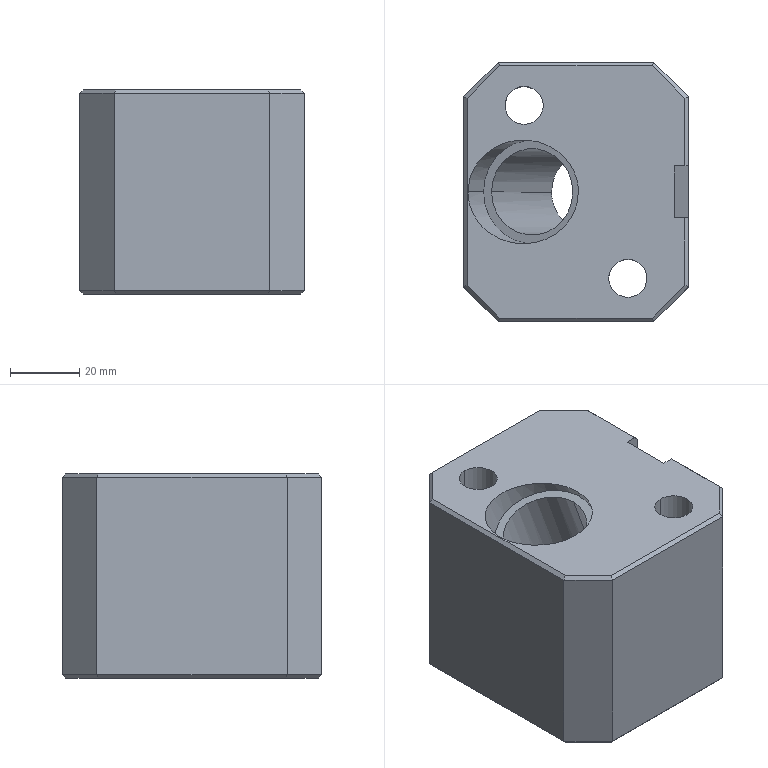Part | Creo | 3 solids | 49 faces | box 65 x 75 x 59 mm | volume 228073 mm3 | plane 33 | cylinder 16 | commonest cylinder face diameters 11 x4 18 x4 11.98 x2 12 x2 25 x2 30 x2
STEP:
#1=CARTESIAN_POINT('',(284.936,-85.497,48.));
#2=VERTEX_POINT('',#1);
#3=CARTESIAN_POINT('',(274.936,-75.497,48.));
#4=VERTEX_POINT('',#3);
#5=CARTESIAN_POINT('',(284.936,-85.497,48.));
#6=DIRECTION('',(-0.7071,0.7071,0.));
#7=VECTOR('',#6,14.142);
#8=LINE('',#5,#7);
#9=EDGE_CURVE('',#2,#4,#8,.T.);
#10=ORIENTED_EDGE('',*,*,#9,.T.);
#11=CARTESIAN_POINT('',(274.936,-75.497,-9.));
#12=VERTEX_POINT('',#11);
#13=CARTESIAN_POINT('',(274.936,-75.497,-9.));
#14=DIRECTION('',(0.,0.,1.));
#15=VECTOR('',#14,57.);
#16=LINE('',#13,#15);
#17=EDGE_CURVE('',#12,#4,#16,.T.);
#18=ORIENTED_EDGE('',*,*,#17,.F.);
#19=CARTESIAN_POINT('',(284.936,-85.497,-9.));
#20=VERTEX_POINT('',#19);
#21=CARTESIAN_POINT('',(274.936,-75.497,-9.));
#22=DIRECTION('',(0.7071,-0.7071,0.));
#23=VECTOR('',#22,14.142);
#24=LINE('',#21,#23);
#25=EDGE_CURVE('',#12,#20,#24,.T.);
#26=ORIENTED_EDGE('',*,*,#25,.T.);
#27=CARTESIAN_POINT('',(284.936,-85.497,48.));
#28=DIRECTION('',(0.,0.,-1.));
#29=VECTOR('',#28,57.);
#30=LINE('',#27,#29);
#31=EDGE_CURVE('',#2,#20,#30,.T.);
#32=ORIENTED_EDGE('',*,*,#31,.F.);
#33=EDGE_LOOP('',(#10,#18,#26,#32));
#34=FACE_OUTER_BOUND('',#33,.F.);
#35=CARTESIAN_POINT('',(274.936,-75.497,-66.89));
#36=DIRECTION('',(0.7071,0.7071,0.));
#37=DIRECTION('',(0.,0.,1.));
#38=AXIS2_PLACEMENT_3D('',#35,#36,#37);
#39=PLANE('',#38);
#40=ADVANCED_FACE('',(#34),#39,.T.);
#41=CARTESIAN_POINT('',(283.936,-85.911,49.));
#42=VERTEX_POINT('',#41);
#43=CARTESIAN_POINT('',(274.522,-76.497,49.));
#44=VERTEX_POINT('',#43);
#45=CARTESIAN_POINT('',(283.936,-85.911,49.));
#46=DIRECTION('',(-0.7071,0.7071,0.));
#47=VECTOR('',#46,13.314);
#48=LINE('',#45,#47);
#49=EDGE_CURVE('',#42,#44,#48,.T.);
#50=ORIENTED_EDGE('',*,*,#49,.T.);
#51=CARTESIAN_POINT('',(274.936,-75.497,48.));
#52=DIRECTION('',(-0.2811,-0.6786,0.6786));
#53=VECTOR('',#52,1.474);
#54=LINE('',#51,#53);
#55=EDGE_CURVE('',#4,#44,#54,.T.);
#56=ORIENTED_EDGE('',*,*,#55,.F.);
#57=ORIENTED_EDGE('',*,*,#9,.F.);
#58=CARTESIAN_POINT('',(284.936,-85.497,48.));
#59=DIRECTION('',(-0.6786,-0.2811,0.6786));
#60=VECTOR('',#59,1.474);
#61=LINE('',#58,#60);
#62=EDGE_CURVE('',#2,#42,#61,.T.);
#63=ORIENTED_EDGE('',*,*,#62,.T.);
#64=EDGE_LOOP('',(#50,#56,#57,#63));
#65=FACE_OUTER_BOUND('',#64,.F.);
#66=CARTESIAN_POINT('',(92.209,105.815,49.));
#67=DIRECTION('',(-0.5,-0.5,-0.7071));
#68=DIRECTION('',(-0.7071,0.7071,0.));
#69=AXIS2_PLACEMENT_3D('',#66,#67,#68);
#70=PLANE('',#69);
#71=ADVANCED_FACE('',(#65),#70,.F.);
#72=CARTESIAN_POINT('',(283.936,-120.497,49.));
#73=VERTEX_POINT('',#72);
#74=CARTESIAN_POINT('',(280.852,-120.497,49.));
#75=VERTEX_POINT('',#74);
#76=CARTESIAN_POINT('',(283.936,-120.497,49.));
#77=DIRECTION('',(-1.,0.,0.));
#78=VECTOR('',#77,3.083);
#79=LINE('',#76,#78);
#80=EDGE_CURVE('',#73,#75,#79,.T.);
#81=ORIENTED_EDGE('',*,*,#80,.F.);
#82=CARTESIAN_POINT('',(283.936,-140.083,49.));
#83=VERTEX_POINT('',#82);
#84=CARTESIAN_POINT('',(283.936,-120.497,49.));
#85=DIRECTION('',(0.,-1.,0.));
#86=VECTOR('',#85,19.586);
#87=LINE('',#84,#86);
#88=EDGE_CURVE('',#73,#83,#87,.T.);
#89=ORIENTED_EDGE('',*,*,#88,.T.);
#90=CARTESIAN_POINT('',(274.522,-149.497,49.));
#91=VERTEX_POINT('',#90);
#92=CARTESIAN_POINT('',(274.522,-149.497,49.));
#93=DIRECTION('',(0.7071,0.7071,0.));
#94=VECTOR('',#93,13.314);
#95=LINE('',#92,#94);
#96=EDGE_CURVE('',#91,#83,#95,.T.);
#97=ORIENTED_EDGE('',*,*,#96,.F.);
#98=CARTESIAN_POINT('',(230.35,-149.497,49.));
#99=VERTEX_POINT('',#98);
#100=CARTESIAN_POINT('',(274.522,-149.497,49.));
#101=DIRECTION('',(-1.,0.,0.));
#102=VECTOR('',#101,44.172);
#103=LINE('',#100,#102);
#104=EDGE_CURVE('',#91,#99,#103,.T.);
#105=ORIENTED_EDGE('',*,*,#104,.T.);
#106=CARTESIAN_POINT('',(220.936,-140.083,49.));
#107=VERTEX_POINT('',#106);
#108=CARTESIAN_POINT('',(220.936,-140.083,49.));
#109=DIRECTION('',(0.7071,-0.7071,0.));
#110=VECTOR('',#109,13.314);
#111=LINE('',#108,#110);
#112=EDGE_CURVE('',#107,#99,#111,.T.);
#113=ORIENTED_EDGE('',*,*,#112,.F.);
#114=CARTESIAN_POINT('',(220.936,-85.911,49.));
#115=VERTEX_POINT('',#114);
#116=CARTESIAN_POINT('',(220.936,-140.083,49.));
#117=DIRECTION('',(0.,1.,0.));
#118=VECTOR('',#117,54.172);
#119=LINE('',#116,#118);
#120=EDGE_CURVE('',#107,#115,#119,.T.);
#121=ORIENTED_EDGE('',*,*,#120,.T.);
#122=CARTESIAN_POINT('',(230.35,-76.497,49.));
#123=VERTEX_POINT('',#122);
#124=CARTESIAN_POINT('',(230.35,-76.497,49.));
#125=DIRECTION('',(-0.7071,-0.7071,0.));
#126=VECTOR('',#125,13.314);
#127=LINE('',#124,#126);
#128=EDGE_CURVE('',#123,#115,#127,.T.);
#129=ORIENTED_EDGE('',*,*,#128,.F.);
#130=CARTESIAN_POINT('',(230.35,-76.497,49.));
#131=DIRECTION('',(1.,0.,0.));
#132=VECTOR('',#131,44.172);
#133=LINE('',#130,#132);
#134=EDGE_CURVE('',#123,#44,#133,.T.);
#135=ORIENTED_EDGE('',*,*,#134,.T.);
#136=ORIENTED_EDGE('',*,*,#49,.F.);
#137=CARTESIAN_POINT('',(283.936,-105.497,49.));
#138=VERTEX_POINT('',#137);
#139=CARTESIAN_POINT('',(283.936,-85.911,49.));
#140=DIRECTION('',(0.,-1.,0.));
#141=VECTOR('',#140,19.586);
#142=LINE('',#139,#141);
#143=EDGE_CURVE('',#42,#138,#142,.T.);
#144=ORIENTED_EDGE('',*,*,#143,.T.);
#145=CARTESIAN_POINT('',(280.852,-105.497,49.));
#146=VERTEX_POINT('',#145);
#147=CARTESIAN_POINT('',(280.852,-105.497,49.));
#148=DIRECTION('',(1.,0.,0.));
#149=VECTOR('',#148,3.083);
#150=LINE('',#147,#149);
#151=EDGE_CURVE('',#146,#138,#150,.T.);
#152=ORIENTED_EDGE('',*,*,#151,.F.);
#153=CARTESIAN_POINT('',(280.852,-120.497,49.));
#154=DIRECTION('',(0.,1.,0.));
#155=VECTOR('',#154,15.);
#156=LINE('',#153,#155);
#157=EDGE_CURVE('',#75,#146,#156,.T.);
#158=ORIENTED_EDGE('',*,*,#157,.F.);
#159=EDGE_LOOP('',(#81,#89,#97,#105,#113,#121,#129,#135,#136,#144,#152,#158));
#160=FACE_OUTER_BOUND('',#159,.F.);
#161=CARTESIAN_POINT('',(237.436,-82.497,49.));
#162=VERTEX_POINT('',#161);
#163=CARTESIAN_POINT('',(237.436,-93.497,49.));
#164=VERTEX_POINT('',#163);
#165=CARTESIAN_POINT('',(237.436,-87.997,49.));
#166=DIRECTION('',(0.,0.,-1.));
#167=DIRECTION('',(0.,1.,0.));
#168=AXIS2_PLACEMENT_3D('',#165,#166,#167);
#169=CIRCLE('',#168,5.5);
#170=EDGE_CURVE('',#162,#164,#169,.T.);
#171=ORIENTED_EDGE('',*,*,#170,.F.);
#172=CARTESIAN_POINT('',(237.436,-87.997,49.));
#173=DIRECTION('',(0.,0.,-1.));
#174=DIRECTION('',(0.,-1.,0.));
#175=AXIS2_PLACEMENT_3D('',#172,#173,#174);
#176=CIRCLE('',#175,5.5);
#177=EDGE_CURVE('',#164,#162,#176,.T.);
#178=ORIENTED_EDGE('',*,*,#177,.F.);
#179=EDGE_LOOP('',(#171,#178));
#180=FACE_BOUND('',#179,.F.);
#181=CARTESIAN_POINT('',(267.436,-132.497,49.));
#182=VERTEX_POINT('',#181);
#183=CARTESIAN_POINT('',(267.436,-143.497,49.));
#184=VERTEX_POINT('',#183);
#185=CARTESIAN_POINT('',(267.436,-137.997,49.));
#186=DIRECTION('',(0.,0.,-1.));
#187=DIRECTION('',(0.,1.,0.));
#188=AXIS2_PLACEMENT_3D('',#185,#186,#187);
#189=CIRCLE('',#188,5.5);
#190=EDGE_CURVE('',#182,#184,#189,.T.);
#191=ORIENTED_EDGE('',*,*,#190,.F.);
#192=CARTESIAN_POINT('',(267.436,-137.997,49.));
#193=DIRECTION('',(0.,0.,-1.));
#194=DIRECTION('',(0.,-1.,0.));
#195=AXIS2_PLACEMENT_3D('',#192,#193,#194);
#196=CIRCLE('',#195,5.5);
#197=EDGE_CURVE('',#184,#182,#196,.T.);
#198=ORIENTED_EDGE('',*,*,#197,.F.);
#199=EDGE_LOOP('',(#191,#198));
#200=FACE_BOUND('',#199,.F.);
#201=CARTESIAN_POINT('',(253.139,-113.005,49.));
#202=VERTEX_POINT('',#201);
#203=CARTESIAN_POINT('',(221.214,-113.005,49.));
#204=VERTEX_POINT('',#203);
#205=CARTESIAN_POINT('',(253.139,-113.005,49.));
#206=CARTESIAN_POINT('',(253.139,-114.772,49.));
#207=CARTESIAN_POINT('',(252.458,-118.593,49.));
#208=CARTESIAN_POINT('',(249.41,-123.034,49.));
#209=CARTESIAN_POINT('',(245.963,-125.654,49.));
#210=CARTESIAN_POINT('',(243.07,-127.052,49.));
#211=CARTESIAN_POINT('',(240.57,-127.715,49.));
#212=CARTESIAN_POINT('',(238.602,-127.966,49.));
#213=CARTESIAN_POINT('',(237.177,-128.024,49.));
#214=CARTESIAN_POINT('',(235.751,-127.966,49.));
#215=CARTESIAN_POINT('',(233.783,-127.715,49.));
#216=CARTESIAN_POINT('',(231.283,-127.052,49.));
#217=CARTESIAN_POINT('',(228.39,-125.654,49.));
#218=CARTESIAN_POINT('',(224.943,-123.034,49.));
#219=CARTESIAN_POINT('',(221.895,-118.593,49.));
#220=CARTESIAN_POINT('',(221.214,-114.772,49.));
#221=CARTESIAN_POINT('',(221.214,-113.005,49.));
#222=B_SPLINE_CURVE_WITH_KNOTS('',3,(#205,#206,#207,#208,#209,#210,#211,#212,#213,#214,#215,#216,#217,#218,#219,#220,#221),.UNSPECIFIED.,.F.,.F.,(4,1,1,1,1,1,1,1,1,1,1,1,1,1,4),(0.,0.125,0.25,0.3125,0.375,0.4375,0.4688,0.5,0.5312,0.5625,0.625,0.6875,0.75,0.875,1.),.UNSPECIFIED.);
#223=EDGE_CURVE('',#202,#204,#222,.T.);
#224=ORIENTED_EDGE('',*,*,#223,.F.);
#225=CARTESIAN_POINT('',(221.214,-113.005,49.));
#226=CARTESIAN_POINT('',(221.214,-111.237,49.));
#227=CARTESIAN_POINT('',(221.895,-107.416,49.));
#228=CARTESIAN_POINT('',(224.943,-102.975,49.));
#229=CARTESIAN_POINT('',(228.39,-100.355,49.));
#230=CARTESIAN_POINT('',(231.283,-98.958,49.));
#231=CARTESIAN_POINT('',(233.783,-98.294,49.));
#232=CARTESIAN_POINT('',(235.751,-98.044,49.));
#233=CARTESIAN_POINT('',(237.177,-97.985,49.));
#234=CARTESIAN_POINT('',(238.602,-98.044,49.));
#235=CARTESIAN_POINT('',(240.57,-98.294,49.));
#236=CARTESIAN_POINT('',(243.07,-98.958,49.));
#237=CARTESIAN_POINT('',(245.963,-100.355,49.));
#238=CARTESIAN_POINT('',(249.41,-102.975,49.));
#239=CARTESIAN_POINT('',(252.458,-107.416,49.));
#240=CARTESIAN_POINT('',(253.139,-111.237,49.));
#241=CARTESIAN_POINT('',(253.139,-113.005,49.));
#242=B_SPLINE_CURVE_WITH_KNOTS('',3,(#225,#226,#227,#228,#229,#230,#231,#232,#233,#234,#235,#236,#237,#238,#239,#240,#241),.UNSPECIFIED.,.F.,.F.,(4,1,1,1,1,1,1,1,1,1,1,1,1,1,4),(0.,0.125,0.25,0.3125,0.375,0.4375,0.4688,0.5,0.5312,0.5625,0.625,0.6875,0.75,0.875,1.),.UNSPECIFIED.);
#243=EDGE_CURVE('',#204,#202,#242,.T.);
#244=ORIENTED_EDGE('',*,*,#243,.F.);
#245=EDGE_LOOP('',(#224,#244));
#246=FACE_BOUND('',#245,.F.);
#247=CARTESIAN_POINT('',(239.333,252.939,49.));
#248=DIRECTION('',(0.,0.,1.));
#249=DIRECTION('',(0.,-1.,0.));
#250=AXIS2_PLACEMENT_3D('',#247,#248,#249);
#251=PLANE('',#250);
#252=ADVANCED_FACE('',(#160,#180,#200,#246),#251,.T.);
#253=ORIENTED_EDGE('',*,*,#80,.T.);
#254=CARTESIAN_POINT('',(284.936,-120.497,37.781));
#255=VERTEX_POINT('',#254);
#256=CARTESIAN_POINT('',(284.936,-120.497,37.781));
#257=DIRECTION('',(-0.342,0.,0.9397));
#258=VECTOR('',#257,11.939);
#259=LINE('',#256,#258);
#260=EDGE_CURVE('',#255,#75,#259,.T.);
#261=ORIENTED_EDGE('',*,*,#260,.F.);
#262=CARTESIAN_POINT('',(284.936,-120.497,48.));
#263=VERTEX_POINT('',#262);
#264=CARTESIAN_POINT('',(284.936,-120.497,37.781));
#265=DIRECTION('',(0.,0.,1.));
#266=VECTOR('',#265,10.219);
#267=LINE('',#264,#266);
#268=EDGE_CURVE('',#255,#263,#267,.T.);
#269=ORIENTED_EDGE('',*,*,#268,.T.);
#270=CARTESIAN_POINT('',(283.936,-120.497,49.));
#271=DIRECTION('',(0.7071,0.,-0.7071));
#272=VECTOR('',#271,1.414);
#273=LINE('',#270,#272);
#274=EDGE_CURVE('',#73,#263,#273,.T.);
#275=ORIENTED_EDGE('',*,*,#274,.F.);
#276=EDGE_LOOP('',(#253,#261,#269,#275));
#277=FACE_OUTER_BOUND('',#276,.F.);
#278=CARTESIAN_POINT('',(301.613,-120.497,-2.93));
#279=DIRECTION('',(0.,-1.,0.));
#280=DIRECTION('',(0.,0.,-1.));
#281=AXIS2_PLACEMENT_3D('',#278,#279,#280);
#282=PLANE('',#281);
#283=ADVANCED_FACE('',(#277),#282,.F.);
#284=ORIENTED_EDGE('',*,*,#157,.T.);
#285=CARTESIAN_POINT('',(284.936,-105.497,37.781));
#286=VERTEX_POINT('',#285);
#287=CARTESIAN_POINT('',(280.852,-105.497,49.));
#288=DIRECTION('',(0.342,0.,-0.9397));
#289=VECTOR('',#288,11.939);
#290=LINE('',#287,#289);
#291=EDGE_CURVE('',#146,#286,#290,.T.);
#292=ORIENTED_EDGE('',*,*,#291,.T.);
#293=CARTESIAN_POINT('',(284.936,-105.497,37.781));
#294=DIRECTION('',(0.,-1.,0.));
#295=VECTOR('',#294,15.);
#296=LINE('',#293,#295);
#297=EDGE_CURVE('',#286,#255,#296,.T.);
#298=ORIENTED_EDGE('',*,*,#297,.T.);
#299=ORIENTED_EDGE('',*,*,#260,.T.);
#300=EDGE_LOOP('',(#284,#292,#298,#299));
#301=FACE_OUTER_BOUND('',#300,.F.);
#302=CARTESIAN_POINT('',(299.971,-112.997,-3.528));
#303=DIRECTION('',(-0.9397,0.,-0.342));
#304=DIRECTION('',(-0.342,0.,0.9397));
#305=AXIS2_PLACEMENT_3D('',#302,#303,#304);
#306=PLANE('',#305);
#307=ADVANCED_FACE('',(#301),#306,.F.);
#308=ORIENTED_EDGE('',*,*,#151,.T.);
#309=CARTESIAN_POINT('',(284.936,-105.497,48.));
#310=VERTEX_POINT('',#309);
#311=CARTESIAN_POINT('',(284.936,-105.497,48.));
#312=DIRECTION('',(-0.7071,0.,0.7071));
#313=VECTOR('',#312,1.414);
#314=LINE('',#311,#313);
#315=EDGE_CURVE('',#310,#138,#314,.T.);
#316=ORIENTED_EDGE('',*,*,#315,.F.);
#317=CARTESIAN_POINT('',(284.936,-105.497,48.));
#318=DIRECTION('',(0.,0.,-1.));
#319=VECTOR('',#318,10.219);
#320=LINE('',#317,#319);
#321=EDGE_CURVE('',#310,#286,#320,.T.);
#322=ORIENTED_EDGE('',*,*,#321,.T.);
#323=ORIENTED_EDGE('',*,*,#291,.F.);
#324=EDGE_LOOP('',(#308,#316,#322,#323));
#325=FACE_OUTER_BOUND('',#324,.F.);
#326=CARTESIAN_POINT('',(301.613,-105.497,-2.93));
#327=DIRECTION('',(0.,1.,0.));
#328=DIRECTION('',(0.,0.,1.));
#329=AXIS2_PLACEMENT_3D('',#326,#327,#328);
#330=PLANE('',#329);
#331=ADVANCED_FACE('',(#325),#330,.F.);
#332=ORIENTED_EDGE('',*,*,#315,.T.);
#333=ORIENTED_EDGE('',*,*,#143,.F.);
#334=ORIENTED_EDGE('',*,*,#62,.F.);
#335=CARTESIAN_POINT('',(284.936,-105.497,48.));
#336=DIRECTION('',(0.,1.,0.));
#337=VECTOR('',#336,20.);
#338=LINE('',#335,#337);
#339=EDGE_CURVE('',#310,#2,#338,.T.);
#340=ORIENTED_EDGE('',*,*,#339,.F.);
#341=EDGE_LOOP('',(#332,#333,#334,#340));
#342=FACE_OUTER_BOUND('',#341,.F.);
#343=CARTESIAN_POINT('',(283.936,252.939,49.));
#344=DIRECTION('',(-0.7071,0.,-0.7071));
#345=DIRECTION('',(0.,1.,0.));
#346=AXIS2_PLACEMENT_3D('',#343,#344,#345);
#347=PLANE('',#346);
#348=ADVANCED_FACE('',(#342),#347,.F.);
#349=ORIENTED_EDGE('',*,*,#268,.F.);
#350=ORIENTED_EDGE('',*,*,#297,.F.);
#351=ORIENTED_EDGE('',*,*,#321,.F.);
#352=ORIENTED_EDGE('',*,*,#339,.T.);
#353=ORIENTED_EDGE('',*,*,#31,.T.);
#354=CARTESIAN_POINT('',(284.936,-140.497,-9.));
#355=VERTEX_POINT('',#354);
#356=CARTESIAN_POINT('',(284.936,-85.497,-9.));
#357=DIRECTION('',(0.,-1.,0.));
#358=VECTOR('',#357,55.);
#359=LINE('',#356,#358);
#360=EDGE_CURVE('',#20,#355,#359,.T.);
#361=ORIENTED_EDGE('',*,*,#360,.T.);
#362=CARTESIAN_POINT('',(284.936,-140.497,48.));
#363=VERTEX_POINT('',#362);
#364=CARTESIAN_POINT('',(284.936,-140.497,-9.));
#365=DIRECTION('',(0.,0.,1.));
#366=VECTOR('',#365,57.);
#367=LINE('',#364,#366);
#368=EDGE_CURVE('',#355,#363,#367,.T.);
#369=ORIENTED_EDGE('',*,*,#368,.T.);
#370=CARTESIAN_POINT('',(284.936,-140.497,48.));
#371=DIRECTION('',(0.,1.,0.));
#372=VECTOR('',#371,20.);
#373=LINE('',#370,#372);
#374=EDGE_CURVE('',#363,#263,#373,.T.);
#375=ORIENTED_EDGE('',*,*,#374,.T.);
#376=EDGE_LOOP('',(#349,#350,#351,#352,#353,#361,#369,#375));
#377=FACE_OUTER_BOUND('',#376,.F.);
#378=CARTESIAN_POINT('',(284.936,77.,-20.39));
#379=DIRECTION('',(1.,0.,0.));
#380=DIRECTION('',(0.,0.,-1.));
#381=AXIS2_PLACEMENT_3D('',#378,#379,#380);
#382=PLANE('',#381);
#383=ADVANCED_FACE('',(#377),#382,.T.);
#384=CARTESIAN_POINT('',(283.936,-140.083,-10.));
#385=VERTEX_POINT('',#384);
#386=CARTESIAN_POINT('',(283.936,-140.083,-10.));
#387=DIRECTION('',(0.6786,-0.2811,0.6786));
#388=VECTOR('',#387,1.474);
#389=LINE('',#386,#388);
#390=EDGE_CURVE('',#385,#355,#389,.T.);
#391=ORIENTED_EDGE('',*,*,#390,.T.);
#392=ORIENTED_EDGE('',*,*,#360,.F.);
#393=CARTESIAN_POINT('',(283.936,-85.911,-10.));
#394=VERTEX_POINT('',#393);
#395=CARTESIAN_POINT('',(283.936,-85.911,-10.));
#396=DIRECTION('',(0.6786,0.2811,0.6786));
#397=VECTOR('',#396,1.474);
#398=LINE('',#395,#397);
#399=EDGE_CURVE('',#394,#20,#398,.T.);
#400=ORIENTED_EDGE('',*,*,#399,.F.);
#401=CARTESIAN_POINT('',(283.936,-140.083,-10.));
#402=DIRECTION('',(0.,1.,0.));
#403=VECTOR('',#402,54.172);
#404=LINE('',#401,#403);
#405=EDGE_CURVE('',#385,#394,#404,.T.);
#406=ORIENTED_EDGE('',*,*,#405,.F.);
#407=EDGE_LOOP('',(#391,#392,#400,#406));
#408=FACE_OUTER_BOUND('',#407,.F.);
#409=CARTESIAN_POINT('',(284.936,77.,-9.));
#410=DIRECTION('',(0.7071,0.,-0.7071));
#411=DIRECTION('',(0.,-1.,0.));
#412=AXIS2_PLACEMENT_3D('',#409,#410,#411);
#413=PLANE('',#412);
#414=ADVANCED_FACE('',(#408),#413,.T.);
#415=CARTESIAN_POINT('',(274.522,-149.497,-10.));
#416=VERTEX_POINT('',#415);
#417=CARTESIAN_POINT('',(274.936,-150.497,-9.));
#418=VERTEX_POINT('',#417);
#419=CARTESIAN_POINT('',(274.522,-149.497,-10.));
#420=DIRECTION('',(0.2811,-0.6786,0.6786));
#421=VECTOR('',#420,1.474);
#422=LINE('',#419,#421);
#423=EDGE_CURVE('',#416,#418,#422,.T.);
#424=ORIENTED_EDGE('',*,*,#423,.T.);
#425=CARTESIAN_POINT('',(284.936,-140.497,-9.));
#426=DIRECTION('',(-0.7071,-0.7071,0.));
#427=VECTOR('',#426,14.142);
#428=LINE('',#425,#427);
#429=EDGE_CURVE('',#355,#418,#428,.T.);
#430=ORIENTED_EDGE('',*,*,#429,.F.);
#431=ORIENTED_EDGE('',*,*,#390,.F.);
#432=CARTESIAN_POINT('',(283.936,-140.083,-10.));
#433=DIRECTION('',(-0.7071,-0.7071,0.));
#434=VECTOR('',#433,13.314);
#435=LINE('',#432,#434);
#436=EDGE_CURVE('',#385,#416,#435,.T.);
#437=ORIENTED_EDGE('',*,*,#436,.T.);
#438=EDGE_LOOP('',(#424,#430,#431,#437));
#439=FACE_OUTER_BOUND('',#438,.F.);
#440=CARTESIAN_POINT('',(-154.521,-578.54,-10.));
#441=DIRECTION('',(-0.5,0.5,0.7071));
#442=DIRECTION('',(-0.7071,-0.7071,0.));
#443=AXIS2_PLACEMENT_3D('',#440,#441,#442);
#444=PLANE('',#443);
#445=ADVANCED_FACE('',(#439),#444,.F.);
#446=CARTESIAN_POINT('',(230.35,-149.497,-10.));
#447=VERTEX_POINT('',#446);
#448=CARTESIAN_POINT('',(229.936,-150.497,-9.));
#449=VERTEX_POINT('',#448);
#450=CARTESIAN_POINT('',(230.35,-149.497,-10.));
#451=DIRECTION('',(-0.2811,-0.6786,0.6786));
#452=VECTOR('',#451,1.474);
#453=LINE('',#450,#452);
#454=EDGE_CURVE('',#447,#449,#453,.T.);
#455=ORIENTED_EDGE('',*,*,#454,.T.);
#456=CARTESIAN_POINT('',(274.936,-150.497,-9.));
#457=DIRECTION('',(-1.,0.,0.));
#458=VECTOR('',#457,45.);
#459=LINE('',#456,#458);
#460=EDGE_CURVE('',#418,#449,#459,.T.);
#461=ORIENTED_EDGE('',*,*,#460,.F.);
#462=ORIENTED_EDGE('',*,*,#423,.F.);
#463=CARTESIAN_POINT('',(230.35,-149.497,-10.));
#464=DIRECTION('',(1.,0.,0.));
#465=VECTOR('',#464,44.172);
#466=LINE('',#463,#465);
#467=EDGE_CURVE('',#447,#416,#466,.T.);
#468=ORIENTED_EDGE('',*,*,#467,.F.);
#469=EDGE_LOOP('',(#455,#461,#462,#468));
#470=FACE_OUTER_BOUND('',#469,.F.);
#471=CARTESIAN_POINT('',(-589.064,-149.497,-10.));
#472=DIRECTION('',(0.,-0.7071,-0.7071));
#473=DIRECTION('',(1.,0.,0.));
#474=AXIS2_PLACEMENT_3D('',#471,#472,#473);
#475=PLANE('',#474);
#476=ADVANCED_FACE('',(#470),#475,.T.);
#477=CARTESIAN_POINT('',(219.936,-140.497,-9.));
#478=VERTEX_POINT('',#477);
#479=CARTESIAN_POINT('',(229.936,-150.497,-9.));
#480=DIRECTION('',(-0.7071,0.7071,0.));
#481=VECTOR('',#480,14.142);
#482=LINE('',#479,#481);
#483=EDGE_CURVE('',#449,#478,#482,.T.);
#484=ORIENTED_EDGE('',*,*,#483,.F.);
#485=ORIENTED_EDGE('',*,*,#454,.F.);
#486=CARTESIAN_POINT('',(220.936,-140.083,-10.));
#487=VERTEX_POINT('',#486);
#488=CARTESIAN_POINT('',(230.35,-149.497,-10.));
#489=DIRECTION('',(-0.7071,0.7071,0.));
#490=VECTOR('',#489,13.314);
#491=LINE('',#488,#490);
#492=EDGE_CURVE('',#447,#487,#491,.T.);
#493=ORIENTED_EDGE('',*,*,#492,.T.);
#494=CARTESIAN_POINT('',(220.936,-140.083,-10.));
#495=DIRECTION('',(-0.6786,-0.2811,0.6786));
#496=VECTOR('',#495,1.474);
#497=LINE('',#494,#496);
#498=EDGE_CURVE('',#487,#478,#497,.T.);
#499=ORIENTED_EDGE('',*,*,#498,.T.);
#500=EDGE_LOOP('',(#484,#485,#493,#499));
#501=FACE_OUTER_BOUND('',#500,.F.);
#502=CARTESIAN_POINT('',(-182.107,262.96,-10.));
#503=DIRECTION('',(0.5,0.5,0.7071));
#504=DIRECTION('',(-0.7071,0.7071,0.));
#505=AXIS2_PLACEMENT_3D('',#502,#503,#504);
#506=PLANE('',#505);
#507=ADVANCED_FACE('',(#501),#506,.F.);
#508=CARTESIAN_POINT('',(219.936,-140.497,48.));
#509=VERTEX_POINT('',#508);
#510=CARTESIAN_POINT('',(219.936,-140.497,48.));
#511=DIRECTION('',(0.,0.,-1.));
#512=VECTOR('',#511,57.);
#513=LINE('',#510,#512);
#514=EDGE_CURVE('',#509,#478,#513,.T.);
#515=ORIENTED_EDGE('',*,*,#514,.F.);
#516=CARTESIAN_POINT('',(229.936,-150.497,48.));
#517=VERTEX_POINT('',#516);
#518=CARTESIAN_POINT('',(219.936,-140.497,48.));
#519=DIRECTION('',(0.7071,-0.7071,0.));
#520=VECTOR('',#519,14.142);
#521=LINE('',#518,#520);
#522=EDGE_CURVE('',#509,#517,#521,.T.);
#523=ORIENTED_EDGE('',*,*,#522,.T.);
#524=CARTESIAN_POINT('',(229.936,-150.497,-9.));
#525=DIRECTION('',(0.,0.,1.));
#526=VECTOR('',#525,57.);
#527=LINE('',#524,#526);
#528=EDGE_CURVE('',#449,#517,#527,.T.);
#529=ORIENTED_EDGE('',*,*,#528,.F.);
#530=ORIENTED_EDGE('',*,*,#483,.T.);
#531=EDGE_LOOP('',(#515,#523,#529,#530));
#532=FACE_OUTER_BOUND('',#531,.F.);
#533=CARTESIAN_POINT('',(219.936,-140.497,19.62));
#534=DIRECTION('',(0.7071,0.7071,0.));
#535=DIRECTION('',(0.,0.,1.));
#536=AXIS2_PLACEMENT_3D('',#533,#534,#535);
#537=PLANE('',#536);
#538=ADVANCED_FACE('',(#532),#537,.F.);
#539=CARTESIAN_POINT('',(219.936,-85.497,-9.));
#540=VERTEX_POINT('',#539);
#541=CARTESIAN_POINT('',(219.936,-85.497,48.));
#542=VERTEX_POINT('',#541);
#543=CARTESIAN_POINT('',(219.936,-85.497,-9.));
#544=DIRECTION('',(0.,0.,1.));
#545=VECTOR('',#544,57.);
#546=LINE('',#543,#545);
#547=EDGE_CURVE('',#540,#542,#546,.T.);
#548=ORIENTED_EDGE('',*,*,#547,.T.);
#549=CARTESIAN_POINT('',(219.936,-85.497,48.));
#550=DIRECTION('',(0.,-1.,0.));
#551=VECTOR('',#550,55.);
#552=LINE('',#549,#551);
#553=EDGE_CURVE('',#542,#509,#552,.T.);
#554=ORIENTED_EDGE('',*,*,#553,.T.);
#555=ORIENTED_EDGE('',*,*,#514,.T.);
#556=CARTESIAN_POINT('',(219.936,-140.497,-9.));
#557=DIRECTION('',(0.,1.,0.));
#558=VECTOR('',#557,55.);
#559=LINE('',#556,#558);
#560=EDGE_CURVE('',#478,#540,#559,.T.);
#561=ORIENTED_EDGE('',*,*,#560,.T.);
#562=EDGE_LOOP('',(#548,#554,#555,#561));
#563=FACE_OUTER_BOUND('',#562,.F.);
#564=CARTESIAN_POINT('',(219.936,165.503,19.62));
#565=DIRECTION('',(-1.,0.,0.));
#566=DIRECTION('',(0.,0.,1.));
#567=AXIS2_PLACEMENT_3D('',#564,#565,#566);
#568=PLANE('',#567);
#569=ADVANCED_FACE('',(#563),#568,.T.);
#570=CARTESIAN_POINT('',(229.936,-75.497,-9.));
#571=VERTEX_POINT('',#570);
#572=CARTESIAN_POINT('',(219.936,-85.497,-9.));
#573=DIRECTION('',(0.7071,0.7071,0.));
#574=VECTOR('',#573,14.142);
#575=LINE('',#572,#574);
#576=EDGE_CURVE('',#540,#571,#575,.T.);
#577=ORIENTED_EDGE('',*,*,#576,.T.);
#578=CARTESIAN_POINT('',(229.936,-75.497,48.));
#579=VERTEX_POINT('',#578);
#580=CARTESIAN_POINT('',(229.936,-75.497,48.));
#581=DIRECTION('',(0.,0.,-1.));
#582=VECTOR('',#581,57.);
#583=LINE('',#580,#582);
#584=EDGE_CURVE('',#579,#571,#583,.T.);
#585=ORIENTED_EDGE('',*,*,#584,.F.);
#586=CARTESIAN_POINT('',(229.936,-75.497,48.));
#587=DIRECTION('',(-0.7071,-0.7071,0.));
#588=VECTOR('',#587,14.142);
#589=LINE('',#586,#588);
#590=EDGE_CURVE('',#579,#542,#589,.T.);
#591=ORIENTED_EDGE('',*,*,#590,.T.);
#592=ORIENTED_EDGE('',*,*,#547,.F.);
#593=EDGE_LOOP('',(#577,#585,#591,#592));
#594=FACE_OUTER_BOUND('',#593,.F.);
#595=CARTESIAN_POINT('',(229.936,-75.497,-66.89));
#596=DIRECTION('',(-0.7071,0.7071,0.));
#597=DIRECTION('',(0.,0.,-1.));
#598=AXIS2_PLACEMENT_3D('',#595,#596,#597);
#599=PLANE('',#598);
#600=ADVANCED_FACE('',(#594),#599,.T.);
#601=CARTESIAN_POINT('',(220.936,-85.911,-10.));
#602=VERTEX_POINT('',#601);
#603=CARTESIAN_POINT('',(230.35,-76.497,-10.));
#604=VERTEX_POINT('',#603);
#605=CARTESIAN_POINT('',(220.936,-85.911,-10.));
#606=DIRECTION('',(0.7071,0.7071,0.));
#607=VECTOR('',#606,13.314);
#608=LINE('',#605,#607);
#609=EDGE_CURVE('',#602,#604,#608,.T.);
#610=ORIENTED_EDGE('',*,*,#609,.T.);
#611=CARTESIAN_POINT('',(229.936,-75.497,-9.));
#612=DIRECTION('',(0.2811,-0.6786,-0.6786));
#613=VECTOR('',#612,1.474);
#614=LINE('',#611,#613);
#615=EDGE_CURVE('',#571,#604,#614,.T.);
#616=ORIENTED_EDGE('',*,*,#615,.F.);
#617=ORIENTED_EDGE('',*,*,#576,.F.);
#618=CARTESIAN_POINT('',(219.936,-85.497,-9.));
#619=DIRECTION('',(0.6786,-0.2811,-0.6786));
#620=VECTOR('',#619,1.474);
#621=LINE('',#618,#620);
#622=EDGE_CURVE('',#540,#602,#621,.T.);
#623=ORIENTED_EDGE('',*,*,#622,.T.);
#624=EDGE_LOOP('',(#610,#616,#617,#623));
#625=FACE_OUTER_BOUND('',#624,.F.);
#626=CARTESIAN_POINT('',(-213.107,-519.954,-10.));
#627=DIRECTION('',(-0.5,0.5,-0.7071));
#628=DIRECTION('',(-0.7071,-0.7071,0.));
#629=AXIS2_PLACEMENT_3D('',#626,#627,#628);
#630=PLANE('',#629);
#631=ADVANCED_FACE('',(#625),#630,.T.);
#632=ORIENTED_EDGE('',*,*,#492,.F.);
#633=ORIENTED_EDGE('',*,*,#467,.T.);
#634=ORIENTED_EDGE('',*,*,#436,.F.);
#635=ORIENTED_EDGE('',*,*,#405,.T.);
#636=CARTESIAN_POINT('',(274.522,-76.497,-10.));
#637=VERTEX_POINT('',#636);
#638=CARTESIAN_POINT('',(274.522,-76.497,-10.));
#639=DIRECTION('',(0.7071,-0.7071,0.));
#640=VECTOR('',#639,13.314);
#641=LINE('',#638,#640);
#642=EDGE_CURVE('',#637,#394,#641,.T.);
#643=ORIENTED_EDGE('',*,*,#642,.F.);
#644=CARTESIAN_POINT('',(274.522,-76.497,-10.));
#645=DIRECTION('',(-1.,0.,0.));
#646=VECTOR('',#645,44.172);
#647=LINE('',#644,#646);
#648=EDGE_CURVE('',#637,#604,#647,.T.);
#649=ORIENTED_EDGE('',*,*,#648,.T.);
#650=ORIENTED_EDGE('',*,*,#609,.F.);
#651=CARTESIAN_POINT('',(220.936,-85.911,-10.));
#652=DIRECTION('',(0.,-1.,0.));
#653=VECTOR('',#652,54.172);
#654=LINE('',#651,#653);
#655=EDGE_CURVE('',#602,#487,#654,.T.);
#656=ORIENTED_EDGE('',*,*,#655,.T.);
#657=EDGE_LOOP('',(#632,#633,#634,#635,#643,#649,#650,#656));
#658=FACE_OUTER_BOUND('',#657,.F.);
#659=CARTESIAN_POINT('',(245.349,-113.005,-10.));
#660=VERTEX_POINT('',#659);
#661=CARTESIAN_POINT('',(271.953,-113.005,-10.));
#662=VERTEX_POINT('',#661);
#663=CARTESIAN_POINT('',(245.349,-113.005,-10.));
#664=CARTESIAN_POINT('',(245.349,-111.532,-10.));
#665=CARTESIAN_POINT('',(245.916,-108.348,-10.));
#666=CARTESIAN_POINT('',(248.457,-104.647,-10.));
#667=CARTESIAN_POINT('',(251.329,-102.463,-10.));
#668=CARTESIAN_POINT('',(253.739,-101.299,-10.));
#669=CARTESIAN_POINT('',(255.822,-100.746,-10.));
#670=CARTESIAN_POINT('',(257.462,-100.537,-10.));
#671=CARTESIAN_POINT('',(258.651,-100.488,-10.));
#672=CARTESIAN_POINT('',(259.839,-100.537,-10.));
#673=CARTESIAN_POINT('',(261.479,-100.746,-10.));
#674=CARTESIAN_POINT('',(263.562,-101.299,-10.));
#675=CARTESIAN_POINT('',(265.973,-102.463,-10.));
#676=CARTESIAN_POINT('',(268.845,-104.647,-10.));
#677=CARTESIAN_POINT('',(271.385,-108.348,-10.));
#678=CARTESIAN_POINT('',(271.953,-111.532,-10.));
#679=CARTESIAN_POINT('',(271.953,-113.005,-10.));
#680=B_SPLINE_CURVE_WITH_KNOTS('',3,(#663,#664,#665,#666,#667,#668,#669,#670,#671,#672,#673,#674,#675,#676,#677,#678,#679),.UNSPECIFIED.,.F.,.F.,(4,1,1,1,1,1,1,1,1,1,1,1,1,1,4),(0.,0.125,0.25,0.3125,0.375,0.4375,0.4688,0.5,0.5312,0.5625,0.625,0.6875,0.75,0.875,1.),.UNSPECIFIED.);
#681=EDGE_CURVE('',#660,#662,#680,.T.);
#682=ORIENTED_EDGE('',*,*,#681,.T.);
#683=CARTESIAN_POINT('',(271.953,-113.005,-10.));
#684=CARTESIAN_POINT('',(271.953,-114.478,-10.));
#685=CARTESIAN_POINT('',(271.385,-117.662,-10.));
#686=CARTESIAN_POINT('',(268.845,-121.362,-10.));
#687=CARTESIAN_POINT('',(265.973,-123.546,-10.));
#688=CARTESIAN_POINT('',(263.562,-124.711,-10.));
#689=CARTESIAN_POINT('',(261.479,-125.263,-10.));
#690=CARTESIAN_POINT('',(259.839,-125.472,-10.));
#691=CARTESIAN_POINT('',(258.651,-125.521,-10.));
#692=CARTESIAN_POINT('',(257.462,-125.472,-10.));
#693=CARTESIAN_POINT('',(255.822,-125.263,-10.));
#694=CARTESIAN_POINT('',(253.739,-124.711,-10.));
#695=CARTESIAN_POINT('',(251.329,-123.546,-10.));
#696=CARTESIAN_POINT('',(248.457,-121.362,-10.));
#697=CARTESIAN_POINT('',(245.916,-117.662,-10.));
#698=CARTESIAN_POINT('',(245.349,-114.478,-10.));
#699=CARTESIAN_POINT('',(245.349,-113.005,-10.));
#700=B_SPLINE_CURVE_WITH_KNOTS('',3,(#683,#684,#685,#686,#687,#688,#689,#690,#691,#692,#693,#694,#695,#696,#697,#698,#699),.UNSPECIFIED.,.F.,.F.,(4,1,1,1,1,1,1,1,1,1,1,1,1,1,4),(0.,0.125,0.25,0.3125,0.375,0.4375,0.4688,0.5,0.5312,0.5625,0.625,0.6875,0.75,0.875,1.),.UNSPECIFIED.);
#701=EDGE_CURVE('',#662,#660,#700,.T.);
#702=ORIENTED_EDGE('',*,*,#701,.T.);
#703=EDGE_LOOP('',(#682,#702));
#704=FACE_BOUND('',#703,.F.);
#705=CARTESIAN_POINT('',(267.436,-128.997,-10.));
#706=VERTEX_POINT('',#705);
#707=CARTESIAN_POINT('',(267.436,-146.997,-10.));
#708=VERTEX_POINT('',#707);
#709=CARTESIAN_POINT('',(267.436,-137.997,-10.));
#710=DIRECTION('',(0.,0.,1.));
#711=DIRECTION('',(0.,1.,0.));
#712=AXIS2_PLACEMENT_3D('',#709,#710,#711);
#713=CIRCLE('',#712,9.);
#714=EDGE_CURVE('',#706,#708,#713,.T.);
#715=ORIENTED_EDGE('',*,*,#714,.F.);
#716=CARTESIAN_POINT('',(267.436,-137.997,-10.));
#717=DIRECTION('',(0.,0.,1.));
#718=DIRECTION('',(0.,-1.,0.));
#719=AXIS2_PLACEMENT_3D('',#716,#717,#718);
#720=CIRCLE('',#719,9.);
#721=EDGE_CURVE('',#708,#706,#720,.T.);
#722=ORIENTED_EDGE('',*,*,#721,.F.);
#723=EDGE_LOOP('',(#715,#722));
#724=FACE_BOUND('',#723,.F.);
#725=CARTESIAN_POINT('',(237.436,-78.997,-10.));
#726=VERTEX_POINT('',#725);
#727=CARTESIAN_POINT('',(237.436,-96.997,-10.));
#728=VERTEX_POINT('',#727);
#729=CARTESIAN_POINT('',(237.436,-87.997,-10.));
#730=DIRECTION('',(0.,0.,1.));
#731=DIRECTION('',(0.,1.,0.));
#732=AXIS2_PLACEMENT_3D('',#729,#730,#731);
#733=CIRCLE('',#732,9.);
#734=EDGE_CURVE('',#726,#728,#733,.T.);
#735=ORIENTED_EDGE('',*,*,#734,.F.);
#736=CARTESIAN_POINT('',(237.436,-87.997,-10.));
#737=DIRECTION('',(0.,0.,1.));
#738=DIRECTION('',(0.,-1.,0.));
#739=AXIS2_PLACEMENT_3D('',#736,#737,#738);
#740=CIRCLE('',#739,9.);
#741=EDGE_CURVE('',#728,#726,#740,.T.);
#742=ORIENTED_EDGE('',*,*,#741,.F.);
#743=EDGE_LOOP('',(#735,#742));
#744=FACE_BOUND('',#743,.F.);
#745=CARTESIAN_POINT('',(-589.064,-143.997,-10.));
#746=DIRECTION('',(0.,0.,1.));
#747=DIRECTION('',(1.,0.,0.));
#748=AXIS2_PLACEMENT_3D('',#745,#746,#747);
#749=PLANE('',#748);
#750=ADVANCED_FACE('',(#658,#704,#724,#744),#749,.F.);
#751=CARTESIAN_POINT('',(228.014,-113.005,37.627));
#752=VERTEX_POINT('',#751);
#753=CARTESIAN_POINT('',(251.506,-113.005,46.178));
#754=VERTEX_POINT('',#753);
#755=CARTESIAN_POINT('',(239.76,-113.005,41.903));
#756=DIRECTION('',(0.342,0.,-0.9397));
#757=DIRECTION('',(-0.9397,0.,-0.342));
#758=AXIS2_PLACEMENT_3D('',#755,#756,#757);
#759=CIRCLE('',#758,12.5);
#760=EDGE_CURVE('',#752,#754,#759,.T.);
#761=ORIENTED_EDGE('',*,*,#760,.T.);
#762=CARTESIAN_POINT('',(251.506,-113.005,46.178));
#763=DIRECTION('',(0.342,0.,-0.9397));
#764=VECTOR('',#763,59.783);
#765=LINE('',#762,#764);
#766=EDGE_CURVE('',#754,#662,#765,.T.);
#767=ORIENTED_EDGE('',*,*,#766,.T.);
#768=ORIENTED_EDGE('',*,*,#681,.F.);
#769=CARTESIAN_POINT('',(228.014,-113.005,37.627));
#770=DIRECTION('',(0.342,0.,-0.9397));
#771=VECTOR('',#770,50.684);
#772=LINE('',#769,#771);
#773=EDGE_CURVE('',#752,#660,#772,.T.);
#774=ORIENTED_EDGE('',*,*,#773,.F.);
#775=EDGE_LOOP('',(#761,#767,#768,#774));
#776=FACE_OUTER_BOUND('',#775,.F.);
#777=CARTESIAN_POINT('',(217.923,-113.005,101.897));
#778=DIRECTION('',(0.342,0.,-0.9397));
#779=DIRECTION('',(0.9397,0.,0.342));
#780=AXIS2_PLACEMENT_3D('',#777,#778,#779);
#781=CYLINDRICAL_SURFACE('',#780,12.5);
#782=ADVANCED_FACE('',(#776),#781,.F.);
#783=CARTESIAN_POINT('',(225.664,-113.005,36.772));
#784=VERTEX_POINT('',#783);
#785=CARTESIAN_POINT('',(253.855,-113.005,47.033));
#786=VERTEX_POINT('',#785);
#787=CARTESIAN_POINT('',(239.76,-113.005,41.903));
#788=DIRECTION('',(-0.342,0.,0.9397));
#789=DIRECTION('',(-0.9397,0.,-0.342));
#790=AXIS2_PLACEMENT_3D('',#787,#788,#789);
#791=CIRCLE('',#790,15.);
#792=EDGE_CURVE('',#784,#786,#791,.T.);
#793=ORIENTED_EDGE('',*,*,#792,.F.);
#794=CARTESIAN_POINT('',(239.76,-113.005,41.903));
#795=DIRECTION('',(-0.342,0.,0.9397));
#796=DIRECTION('',(0.9397,0.,0.342));
#797=AXIS2_PLACEMENT_3D('',#794,#795,#796);
#798=CIRCLE('',#797,15.);
#799=EDGE_CURVE('',#786,#784,#798,.T.);
#800=ORIENTED_EDGE('',*,*,#799,.F.);
#801=EDGE_LOOP('',(#793,#800));
#802=FACE_OUTER_BOUND('',#801,.F.);
#803=ORIENTED_EDGE('',*,*,#760,.F.);
#804=CARTESIAN_POINT('',(239.76,-113.005,41.903));
#805=DIRECTION('',(0.342,0.,-0.9397));
#806=DIRECTION('',(0.9397,0.,0.342));
#807=AXIS2_PLACEMENT_3D('',#804,#805,#806);
#808=CIRCLE('',#807,12.5);
#809=EDGE_CURVE('',#754,#752,#808,.T.);
#810=ORIENTED_EDGE('',*,*,#809,.F.);
#811=EDGE_LOOP('',(#803,#810));
#812=FACE_BOUND('',#811,.F.);
#813=CARTESIAN_POINT('',(239.76,-113.005,41.903));
#814=DIRECTION('',(0.342,0.,-0.9397));
#815=DIRECTION('',(0.9397,0.,0.342));
#816=AXIS2_PLACEMENT_3D('',#813,#814,#815);
#817=PLANE('',#816);
#818=ADVANCED_FACE('',(#802,#812),#817,.F.);
#819=ORIENTED_EDGE('',*,*,#809,.T.);
#820=ORIENTED_EDGE('',*,*,#773,.T.);
#821=ORIENTED_EDGE('',*,*,#701,.F.);
#822=ORIENTED_EDGE('',*,*,#766,.F.);
#823=EDGE_LOOP('',(#819,#820,#821,#822));
#824=FACE_OUTER_BOUND('',#823,.F.);
#825=CARTESIAN_POINT('',(217.923,-113.005,101.897));
#826=DIRECTION('',(0.342,0.,-0.9397));
#827=DIRECTION('',(0.9397,0.,0.342));
#828=AXIS2_PLACEMENT_3D('',#825,#826,#827);
#829=CYLINDRICAL_SURFACE('',#828,12.5);
#830=ADVANCED_FACE('',(#824),#829,.F.);
#831=ORIENTED_EDGE('',*,*,#792,.T.);
#832=CARTESIAN_POINT('',(253.139,-113.005,49.));
#833=DIRECTION('',(0.342,0.,-0.9397));
#834=VECTOR('',#833,2.093);
#835=LINE('',#832,#834);
#836=EDGE_CURVE('',#202,#786,#835,.T.);
#837=ORIENTED_EDGE('',*,*,#836,.F.);
#838=ORIENTED_EDGE('',*,*,#223,.T.);
#839=CARTESIAN_POINT('',(221.214,-113.005,49.));
#840=DIRECTION('',(0.342,0.,-0.9397));
#841=VECTOR('',#840,13.012);
#842=LINE('',#839,#841);
#843=EDGE_CURVE('',#204,#784,#842,.T.);
#844=ORIENTED_EDGE('',*,*,#843,.T.);
#845=EDGE_LOOP('',(#831,#837,#838,#844));
#846=FACE_OUTER_BOUND('',#845,.F.);
#847=CARTESIAN_POINT('',(232.329,-113.005,62.317));
#848=DIRECTION('',(0.342,0.,-0.9397));
#849=DIRECTION('',(0.9397,0.,0.342));
#850=AXIS2_PLACEMENT_3D('',#847,#848,#849);
#851=CYLINDRICAL_SURFACE('',#850,15.);
#852=ADVANCED_FACE('',(#846),#851,.F.);
#853=ORIENTED_EDGE('',*,*,#799,.T.);
#854=ORIENTED_EDGE('',*,*,#843,.F.);
#855=ORIENTED_EDGE('',*,*,#243,.T.);
#856=ORIENTED_EDGE('',*,*,#836,.T.);
#857=EDGE_LOOP('',(#853,#854,#855,#856));
#858=FACE_OUTER_BOUND('',#857,.F.);
#859=CARTESIAN_POINT('',(232.329,-113.005,62.317));
#860=DIRECTION('',(0.342,0.,-0.9397));
#861=DIRECTION('',(0.9397,0.,0.342));
#862=AXIS2_PLACEMENT_3D('',#859,#860,#861);
#863=CYLINDRICAL_SURFACE('',#862,15.);
#864=ADVANCED_FACE('',(#858),#863,.F.);
#865=CARTESIAN_POINT('',(274.936,-75.497,-9.));
#866=DIRECTION('',(-0.2811,-0.6786,-0.6786));
#867=VECTOR('',#866,1.474);
#868=LINE('',#865,#867);
#869=EDGE_CURVE('',#12,#637,#868,.T.);
#870=ORIENTED_EDGE('',*,*,#869,.T.);
#871=ORIENTED_EDGE('',*,*,#642,.T.);
#872=ORIENTED_EDGE('',*,*,#399,.T.);
#873=ORIENTED_EDGE('',*,*,#25,.F.);
#874=EDGE_LOOP('',(#870,#871,#872,#873));
#875=FACE_OUTER_BOUND('',#874,.F.);
#876=CARTESIAN_POINT('',(-123.521,321.546,-10.));
#877=DIRECTION('',(0.5,0.5,-0.7071));
#878=DIRECTION('',(-0.7071,0.7071,0.));
#879=AXIS2_PLACEMENT_3D('',#876,#877,#878);
#880=PLANE('',#879);
#881=ADVANCED_FACE('',(#875),#880,.T.);
#882=ORIENTED_EDGE('',*,*,#615,.T.);
#883=ORIENTED_EDGE('',*,*,#648,.F.);
#884=ORIENTED_EDGE('',*,*,#869,.F.);
#885=CARTESIAN_POINT('',(229.936,-75.497,-9.));
#886=DIRECTION('',(1.,0.,0.));
#887=VECTOR('',#886,45.);
#888=LINE('',#885,#887);
#889=EDGE_CURVE('',#571,#12,#888,.T.);
#890=ORIENTED_EDGE('',*,*,#889,.F.);
#891=EDGE_LOOP('',(#882,#883,#884,#890));
#892=FACE_OUTER_BOUND('',#891,.F.);
#893=CARTESIAN_POINT('',(-589.064,-76.497,-10.));
#894=DIRECTION('',(0.,-0.7071,0.7071));
#895=DIRECTION('',(1.,0.,0.));
#896=AXIS2_PLACEMENT_3D('',#893,#894,#895);
#897=PLANE('',#896);
#898=ADVANCED_FACE('',(#892),#897,.F.);
#899=ORIENTED_EDGE('',*,*,#17,.T.);
#900=CARTESIAN_POINT('',(274.936,-75.497,48.));
#901=DIRECTION('',(-1.,0.,0.));
#902=VECTOR('',#901,45.);
#903=LINE('',#900,#902);
#904=EDGE_CURVE('',#4,#579,#903,.T.);
#905=ORIENTED_EDGE('',*,*,#904,.T.);
#906=ORIENTED_EDGE('',*,*,#584,.T.);
#907=ORIENTED_EDGE('',*,*,#889,.T.);
#908=EDGE_LOOP('',(#899,#905,#906,#907));
#909=FACE_OUTER_BOUND('',#908,.F.);
#910=CARTESIAN_POINT('',(271.052,-75.497,-66.89));
#911=DIRECTION('',(0.,-1.,0.));
#912=DIRECTION('',(0.,0.,1.));
#913=AXIS2_PLACEMENT_3D('',#910,#911,#912);
#914=PLANE('',#913);
#915=ADVANCED_FACE('',(#909),#914,.F.);
#916=ORIENTED_EDGE('',*,*,#55,.T.);
#917=ORIENTED_EDGE('',*,*,#134,.F.);
#918=CARTESIAN_POINT('',(229.936,-75.497,48.));
#919=DIRECTION('',(0.2811,-0.6786,0.6786));
#920=VECTOR('',#919,1.474);
#921=LINE('',#918,#920);
#922=EDGE_CURVE('',#579,#123,#921,.T.);
#923=ORIENTED_EDGE('',*,*,#922,.F.);
#924=ORIENTED_EDGE('',*,*,#904,.F.);
#925=EDGE_LOOP('',(#916,#917,#923,#924));
#926=FACE_OUTER_BOUND('',#925,.F.);
#927=CARTESIAN_POINT('',(239.333,-76.497,49.));
#928=DIRECTION('',(0.,0.7071,0.7071));
#929=DIRECTION('',(1.,0.,0.));
#930=AXIS2_PLACEMENT_3D('',#927,#928,#929);
#931=PLANE('',#930);
#932=ADVANCED_FACE('',(#926),#931,.T.);
#933=ORIENTED_EDGE('',*,*,#922,.T.);
#934=ORIENTED_EDGE('',*,*,#128,.T.);
#935=CARTESIAN_POINT('',(219.936,-85.497,48.));
#936=DIRECTION('',(0.6786,-0.2811,0.6786));
#937=VECTOR('',#936,1.474);
#938=LINE('',#935,#937);
#939=EDGE_CURVE('',#542,#115,#938,.T.);
#940=ORIENTED_EDGE('',*,*,#939,.F.);
#941=ORIENTED_EDGE('',*,*,#590,.F.);
#942=EDGE_LOOP('',(#933,#934,#940,#941));
#943=FACE_OUTER_BOUND('',#942,.F.);
#944=CARTESIAN_POINT('',(399.56,92.713,49.));
#945=DIRECTION('',(0.5,-0.5,-0.7071));
#946=DIRECTION('',(-0.7071,-0.7071,0.));
#947=AXIS2_PLACEMENT_3D('',#944,#945,#946);
#948=PLANE('',#947);
#949=ADVANCED_FACE('',(#943),#948,.F.);
#950=CARTESIAN_POINT('',(219.936,-140.497,48.));
#951=DIRECTION('',(0.6786,0.2811,0.6786));
#952=VECTOR('',#951,1.474);
#953=LINE('',#950,#952);
#954=EDGE_CURVE('',#509,#107,#953,.T.);
#955=ORIENTED_EDGE('',*,*,#954,.F.);
#956=ORIENTED_EDGE('',*,*,#553,.F.);
#957=ORIENTED_EDGE('',*,*,#939,.T.);
#958=ORIENTED_EDGE('',*,*,#120,.F.);
#959=EDGE_LOOP('',(#955,#956,#957,#958));
#960=FACE_OUTER_BOUND('',#959,.F.);
#961=CARTESIAN_POINT('',(219.936,165.503,48.));
#962=DIRECTION('',(0.7071,0.,-0.7071));
#963=DIRECTION('',(0.,1.,0.));
#964=AXIS2_PLACEMENT_3D('',#961,#962,#963);
#965=PLANE('',#964);
#966=ADVANCED_FACE('',(#960),#965,.F.);
#967=ORIENTED_EDGE('',*,*,#954,.T.);
#968=ORIENTED_EDGE('',*,*,#112,.T.);
#969=CARTESIAN_POINT('',(230.35,-149.497,49.));
#970=DIRECTION('',(-0.2811,-0.6786,-0.6786));
#971=VECTOR('',#970,1.474);
#972=LINE('',#969,#971);
#973=EDGE_CURVE('',#99,#517,#972,.T.);
#974=ORIENTED_EDGE('',*,*,#973,.T.);
#975=ORIENTED_EDGE('',*,*,#522,.F.);
#976=EDGE_LOOP('',(#967,#968,#974,#975));
#977=FACE_OUTER_BOUND('',#976,.F.);
#978=CARTESIAN_POINT('',(33.624,47.23,49.));
#979=DIRECTION('',(-0.5,-0.5,0.7071));
#980=DIRECTION('',(-0.7071,0.7071,0.));
#981=AXIS2_PLACEMENT_3D('',#978,#979,#980);
#982=PLANE('',#981);
#983=ADVANCED_FACE('',(#977),#982,.T.);
#984=CARTESIAN_POINT('',(274.936,-150.497,48.));
#985=VERTEX_POINT('',#984);
#986=CARTESIAN_POINT('',(274.522,-149.497,49.));
#987=DIRECTION('',(0.2811,-0.6786,-0.6786));
#988=VECTOR('',#987,1.474);
#989=LINE('',#986,#988);
#990=EDGE_CURVE('',#91,#985,#989,.T.);
#991=ORIENTED_EDGE('',*,*,#990,.T.);
#992=CARTESIAN_POINT('',(229.936,-150.497,48.));
#993=DIRECTION('',(1.,0.,0.));
#994=VECTOR('',#993,45.);
#995=LINE('',#992,#994);
#996=EDGE_CURVE('',#517,#985,#995,.T.);
#997=ORIENTED_EDGE('',*,*,#996,.F.);
#998=ORIENTED_EDGE('',*,*,#973,.F.);
#999=ORIENTED_EDGE('',*,*,#104,.F.);
#1000=EDGE_LOOP('',(#991,#997,#998,#999));
#1001=FACE_OUTER_BOUND('',#1000,.F.);
#1002=CARTESIAN_POINT('',(239.333,-149.497,49.));
#1003=DIRECTION('',(0.,0.7071,-0.7071));
#1004=DIRECTION('',(1.,0.,0.));
#1005=AXIS2_PLACEMENT_3D('',#1002,#1003,#1004);
#1006=PLANE('',#1005);
#1007=ADVANCED_FACE('',(#1001),#1006,.F.);
#1008=CARTESIAN_POINT('',(274.936,-150.497,48.));
#1009=DIRECTION('',(0.7071,0.7071,0.));
#1010=VECTOR('',#1009,14.142);
#1011=LINE('',#1008,#1010);
#1012=EDGE_CURVE('',#985,#363,#1011,.T.);
#1013=ORIENTED_EDGE('',*,*,#1012,.F.);
#1014=ORIENTED_EDGE('',*,*,#990,.F.);
#1015=ORIENTED_EDGE('',*,*,#96,.T.);
#1016=CARTESIAN_POINT('',(283.936,-140.083,49.));
#1017=DIRECTION('',(0.6786,-0.2811,-0.6786));
#1018=VECTOR('',#1017,1.474);
#1019=LINE('',#1016,#1018);
#1020=EDGE_CURVE('',#83,#363,#1019,.T.);
#1021=ORIENTED_EDGE('',*,*,#1020,.T.);
#1022=EDGE_LOOP('',(#1013,#1014,#1015,#1021));
#1023=FACE_OUTER_BOUND('',#1022,.F.);
#1024=CARTESIAN_POINT('',(458.145,34.127,49.));
#1025=DIRECTION('',(0.5,-0.5,0.7071));
#1026=DIRECTION('',(-0.7071,-0.7071,0.));
#1027=AXIS2_PLACEMENT_3D('',#1024,#1025,#1026);
#1028=PLANE('',#1027);
#1029=ADVANCED_FACE('',(#1023),#1028,.T.);
#1030=ORIENTED_EDGE('',*,*,#368,.F.);
#1031=ORIENTED_EDGE('',*,*,#429,.T.);
#1032=CARTESIAN_POINT('',(274.936,-150.497,48.));
#1033=DIRECTION('',(0.,0.,-1.));
#1034=VECTOR('',#1033,57.);
#1035=LINE('',#1032,#1034);
#1036=EDGE_CURVE('',#985,#418,#1035,.T.);
#1037=ORIENTED_EDGE('',*,*,#1036,.F.);
#1038=ORIENTED_EDGE('',*,*,#1012,.T.);
#1039=EDGE_LOOP('',(#1030,#1031,#1037,#1038));
#1040=FACE_OUTER_BOUND('',#1039,.F.);
#1041=CARTESIAN_POINT('',(284.936,-140.497,-20.39));
#1042=DIRECTION('',(-0.7071,0.7071,0.));
#1043=DIRECTION('',(0.,0.,-1.));
#1044=AXIS2_PLACEMENT_3D('',#1041,#1042,#1043);
#1045=PLANE('',#1044);
#1046=ADVANCED_FACE('',(#1040),#1045,.F.);
#1047=ORIENTED_EDGE('',*,*,#528,.T.);
#1048=ORIENTED_EDGE('',*,*,#996,.T.);
#1049=ORIENTED_EDGE('',*,*,#1036,.T.);
#1050=ORIENTED_EDGE('',*,*,#460,.T.);
#1051=EDGE_LOOP('',(#1047,#1048,#1049,#1050));
#1052=FACE_OUTER_BOUND('',#1051,.F.);
#1053=CARTESIAN_POINT('',(224.333,-150.497,49.24));
#1054=DIRECTION('',(0.,-1.,0.));
#1055=DIRECTION('',(0.,0.,-1.));
#1056=AXIS2_PLACEMENT_3D('',#1053,#1054,#1055);
#1057=PLANE('',#1056);
#1058=ADVANCED_FACE('',(#1052),#1057,.T.);
#1059=ORIENTED_EDGE('',*,*,#274,.T.);
#1060=ORIENTED_EDGE('',*,*,#374,.F.);
#1061=ORIENTED_EDGE('',*,*,#1020,.F.);
#1062=ORIENTED_EDGE('',*,*,#88,.F.);
#1063=EDGE_LOOP('',(#1059,#1060,#1061,#1062));
#1064=FACE_OUTER_BOUND('',#1063,.F.);
#1065=CARTESIAN_POINT('',(283.936,252.939,49.));
#1066=DIRECTION('',(-0.7071,0.,-0.7071));
#1067=DIRECTION('',(0.,1.,0.));
#1068=AXIS2_PLACEMENT_3D('',#1065,#1066,#1067);
#1069=PLANE('',#1068);
#1070=ADVANCED_FACE('',(#1064),#1069,.F.);
#1071=ORIENTED_EDGE('',*,*,#498,.F.);
#1072=ORIENTED_EDGE('',*,*,#655,.F.);
#1073=ORIENTED_EDGE('',*,*,#622,.F.);
#1074=ORIENTED_EDGE('',*,*,#560,.F.);
#1075=EDGE_LOOP('',(#1071,#1072,#1073,#1074));
#1076=FACE_OUTER_BOUND('',#1075,.F.);
#1077=CARTESIAN_POINT('',(220.936,-143.997,-10.));
#1078=DIRECTION('',(-0.7071,0.,-0.7071));
#1079=DIRECTION('',(0.,-1.,0.));
#1080=AXIS2_PLACEMENT_3D('',#1077,#1078,#1079);
#1081=PLANE('',#1080);
#1082=ADVANCED_FACE('',(#1076),#1081,.T.);
#1083=CARTESIAN_POINT('',(267.436,-146.997,0.9999));
#1084=VERTEX_POINT('',#1083);
#1085=CARTESIAN_POINT('',(267.436,-128.997,0.9999));
#1086=VERTEX_POINT('',#1085);
#1087=CARTESIAN_POINT('',(267.436,-137.997,0.9999));
#1088=DIRECTION('',(0.,0.,-1.));
#1089=DIRECTION('',(0.,-1.,0.));
#1090=AXIS2_PLACEMENT_3D('',#1087,#1088,#1089);
#1091=CIRCLE('',#1090,9.);
#1092=EDGE_CURVE('',#1084,#1086,#1091,.T.);
#1093=ORIENTED_EDGE('',*,*,#1092,.T.);
#1094=CARTESIAN_POINT('',(267.436,-128.997,-10.));
#1095=DIRECTION('',(0.,0.,1.));
#1096=VECTOR('',#1095,11.);
#1097=LINE('',#1094,#1096);
#1098=EDGE_CURVE('',#706,#1086,#1097,.T.);
#1099=ORIENTED_EDGE('',*,*,#1098,.F.);
#1100=ORIENTED_EDGE('',*,*,#714,.T.);
#1101=CARTESIAN_POINT('',(267.436,-146.997,-10.));
#1102=DIRECTION('',(0.,0.,1.));
#1103=VECTOR('',#1102,11.);
#1104=LINE('',#1101,#1103);
#1105=EDGE_CURVE('',#708,#1084,#1104,.T.);
#1106=ORIENTED_EDGE('',*,*,#1105,.T.);
#1107=EDGE_LOOP('',(#1093,#1099,#1100,#1106));
#1108=FACE_OUTER_BOUND('',#1107,.F.);
#1109=CARTESIAN_POINT('',(267.436,-137.997,-10.));
#1110=DIRECTION('',(0.,0.,1.));
#1111=DIRECTION('',(0.,1.,0.));
#1112=AXIS2_PLACEMENT_3D('',#1109,#1110,#1111);
#1113=CYLINDRICAL_SURFACE('',#1112,9.);
#1114=ADVANCED_FACE('',(#1108),#1113,.F.);
#1115=CARTESIAN_POINT('',(267.436,-137.997,0.9999));
#1116=DIRECTION('',(0.,0.,-1.));
#1117=DIRECTION('',(0.,1.,0.));
#1118=AXIS2_PLACEMENT_3D('',#1115,#1116,#1117);
#1119=CIRCLE('',#1118,9.);
#1120=EDGE_CURVE('',#1086,#1084,#1119,.T.);
#1121=ORIENTED_EDGE('',*,*,#1120,.F.);
#1122=ORIENTED_EDGE('',*,*,#1092,.F.);
#1123=EDGE_LOOP('',(#1121,#1122));
#1124=FACE_OUTER_BOUND('',#1123,.F.);
#1125=CARTESIAN_POINT('',(267.436,-132.497,0.9999));
#1126=VERTEX_POINT('',#1125);
#1127=CARTESIAN_POINT('',(267.436,-143.497,0.9999));
#1128=VERTEX_POINT('',#1127);
#1129=CARTESIAN_POINT('',(267.436,-137.997,0.9999));
#1130=DIRECTION('',(0.,0.,1.));
#1131=DIRECTION('',(0.,1.,0.));
#1132=AXIS2_PLACEMENT_3D('',#1129,#1130,#1131);
#1133=CIRCLE('',#1132,5.5);
#1134=EDGE_CURVE('',#1126,#1128,#1133,.T.);
#1135=ORIENTED_EDGE('',*,*,#1134,.F.);
#1136=CARTESIAN_POINT('',(267.436,-137.997,0.9999));
#1137=DIRECTION('',(0.,0.,1.));
#1138=DIRECTION('',(0.,-1.,0.));
#1139=AXIS2_PLACEMENT_3D('',#1136,#1137,#1138);
#1140=CIRCLE('',#1139,5.5);
#1141=EDGE_CURVE('',#1128,#1126,#1140,.T.);
#1142=ORIENTED_EDGE('',*,*,#1141,.F.);
#1143=EDGE_LOOP('',(#1135,#1142));
#1144=FACE_BOUND('',#1143,.F.);
#1145=CARTESIAN_POINT('',(267.436,-137.997,0.9999));
#1146=DIRECTION('',(0.,0.,1.));
#1147=DIRECTION('',(0.,1.,0.));
#1148=AXIS2_PLACEMENT_3D('',#1145,#1146,#1147);
#1149=PLANE('',#1148);
#1150=ADVANCED_FACE('',(#1124,#1144),#1149,.F.);
#1151=ORIENTED_EDGE('',*,*,#1120,.T.);
#1152=ORIENTED_EDGE('',*,*,#1105,.F.);
#1153=ORIENTED_EDGE('',*,*,#721,.T.);
#1154=ORIENTED_EDGE('',*,*,#1098,.T.);
#1155=EDGE_LOOP('',(#1151,#1152,#1153,#1154));
#1156=FACE_OUTER_BOUND('',#1155,.F.);
#1157=CARTESIAN_POINT('',(267.436,-137.997,-10.));
#1158=DIRECTION('',(0.,0.,1.));
#1159=DIRECTION('',(0.,1.,0.));
#1160=AXIS2_PLACEMENT_3D('',#1157,#1158,#1159);
#1161=CYLINDRICAL_SURFACE('',#1160,9.);
#1162=ADVANCED_FACE('',(#1156),#1161,.F.);
#1163=ORIENTED_EDGE('',*,*,#1134,.T.);
#1164=CARTESIAN_POINT('',(267.436,-143.497,0.9999));
#1165=DIRECTION('',(0.,0.,1.));
#1166=VECTOR('',#1165,48.);
#1167=LINE('',#1164,#1166);
#1168=EDGE_CURVE('',#1128,#184,#1167,.T.);
#1169=ORIENTED_EDGE('',*,*,#1168,.T.);
#1170=ORIENTED_EDGE('',*,*,#197,.T.);
#1171=CARTESIAN_POINT('',(267.436,-132.497,0.9999));
#1172=DIRECTION('',(0.,0.,1.));
#1173=VECTOR('',#1172,48.);
#1174=LINE('',#1171,#1173);
#1175=EDGE_CURVE('',#1126,#182,#1174,.T.);
#1176=ORIENTED_EDGE('',*,*,#1175,.F.);
#1177=EDGE_LOOP('',(#1163,#1169,#1170,#1176));
#1178=FACE_OUTER_BOUND('',#1177,.F.);
#1179=CARTESIAN_POINT('',(267.436,-137.997,-10.));
#1180=DIRECTION('',(0.,0.,1.));
#1181=DIRECTION('',(0.,1.,0.));
#1182=AXIS2_PLACEMENT_3D('',#1179,#1180,#1181);
#1183=CYLINDRICAL_SURFACE('',#1182,5.5);
#1184=ADVANCED_FACE('',(#1178),#1183,.F.);
#1185=ORIENTED_EDGE('',*,*,#1141,.T.);
#1186=ORIENTED_EDGE('',*,*,#1175,.T.);
#1187=ORIENTED_EDGE('',*,*,#190,.T.);
#1188=ORIENTED_EDGE('',*,*,#1168,.F.);
#1189=EDGE_LOOP('',(#1185,#1186,#1187,#1188));
#1190=FACE_OUTER_BOUND('',#1189,.F.);
#1191=CARTESIAN_POINT('',(267.436,-137.997,-10.));
#1192=DIRECTION('',(0.,0.,1.));
#1193=DIRECTION('',(0.,1.,0.));
#1194=AXIS2_PLACEMENT_3D('',#1191,#1192,#1193);
#1195=CYLINDRICAL_SURFACE('',#1194,5.5);
#1196=ADVANCED_FACE('',(#1190),#1195,.F.);
#1197=CARTESIAN_POINT('',(237.436,-96.997,0.9999));
#1198=VERTEX_POINT('',#1197);
#1199=CARTESIAN_POINT('',(237.436,-78.997,0.9999));
#1200=VERTEX_POINT('',#1199);
#1201=CARTESIAN_POINT('',(237.436,-87.997,0.9999));
#1202=DIRECTION('',(0.,0.,-1.));
#1203=DIRECTION('',(0.,-1.,0.));
#1204=AXIS2_PLACEMENT_3D('',#1201,#1202,#1203);
#1205=CIRCLE('',#1204,9.);
#1206=EDGE_CURVE('',#1198,#1200,#1205,.T.);
#1207=ORIENTED_EDGE('',*,*,#1206,.T.);
#1208=CARTESIAN_POINT('',(237.436,-78.997,-10.));
#1209=DIRECTION('',(0.,0.,1.));
#1210=VECTOR('',#1209,11.);
#1211=LINE('',#1208,#1210);
#1212=EDGE_CURVE('',#726,#1200,#1211,.T.);
#1213=ORIENTED_EDGE('',*,*,#1212,.F.);
#1214=ORIENTED_EDGE('',*,*,#734,.T.);
#1215=CARTESIAN_POINT('',(237.436,-96.997,-10.));
#1216=DIRECTION('',(0.,0.,1.));
#1217=VECTOR('',#1216,11.);
#1218=LINE('',#1215,#1217);
#1219=EDGE_CURVE('',#728,#1198,#1218,.T.);
#1220=ORIENTED_EDGE('',*,*,#1219,.T.);
#1221=EDGE_LOOP('',(#1207,#1213,#1214,#1220));
#1222=FACE_OUTER_BOUND('',#1221,.F.);
#1223=CARTESIAN_POINT('',(237.436,-87.997,-10.));
#1224=DIRECTION('',(0.,0.,1.));
#1225=DIRECTION('',(0.,1.,0.));
#1226=AXIS2_PLACEMENT_3D('',#1223,#1224,#1225);
#1227=CYLINDRICAL_SURFACE('',#1226,9.);
#1228=ADVANCED_FACE('',(#1222),#1227,.F.);
#1229=CARTESIAN_POINT('',(237.436,-87.997,0.9999));
#1230=DIRECTION('',(0.,0.,-1.));
#1231=DIRECTION('',(0.,1.,0.));
#1232=AXIS2_PLACEMENT_3D('',#1229,#1230,#1231);
#1233=CIRCLE('',#1232,9.);
#1234=EDGE_CURVE('',#1200,#1198,#1233,.T.);
#1235=ORIENTED_EDGE('',*,*,#1234,.F.);
#1236=ORIENTED_EDGE('',*,*,#1206,.F.);
#1237=EDGE_LOOP('',(#1235,#1236));
#1238=FACE_OUTER_BOUND('',#1237,.F.);
#1239=CARTESIAN_POINT('',(237.436,-82.497,0.9999));
#1240=VERTEX_POINT('',#1239);
#1241=CARTESIAN_POINT('',(237.436,-93.497,0.9999));
#1242=VERTEX_POINT('',#1241);
#1243=CARTESIAN_POINT('',(237.436,-87.997,0.9999));
#1244=DIRECTION('',(0.,0.,1.));
#1245=DIRECTION('',(0.,1.,0.));
#1246=AXIS2_PLACEMENT_3D('',#1243,#1244,#1245);
#1247=CIRCLE('',#1246,5.5);
#1248=EDGE_CURVE('',#1240,#1242,#1247,.T.);
#1249=ORIENTED_EDGE('',*,*,#1248,.F.);
#1250=CARTESIAN_POINT('',(237.436,-87.997,0.9999));
#1251=DIRECTION('',(0.,0.,1.));
#1252=DIRECTION('',(0.,-1.,0.));
#1253=AXIS2_PLACEMENT_3D('',#1250,#1251,#1252);
#1254=CIRCLE('',#1253,5.5);
#1255=EDGE_CURVE('',#1242,#1240,#1254,.T.);
#1256=ORIENTED_EDGE('',*,*,#1255,.F.);
#1257=EDGE_LOOP('',(#1249,#1256));
#1258=FACE_BOUND('',#1257,.F.);
#1259=CARTESIAN_POINT('',(237.436,-87.997,0.9999));
#1260=DIRECTION('',(0.,0.,1.));
#1261=DIRECTION('',(0.,1.,0.));
#1262=AXIS2_PLACEMENT_3D('',#1259,#1260,#1261);
#1263=PLANE('',#1262);
#1264=ADVANCED_FACE('',(#1238,#1258),#1263,.F.);
#1265=ORIENTED_EDGE('',*,*,#1234,.T.);
#1266=ORIENTED_EDGE('',*,*,#1219,.F.);
#1267=ORIENTED_EDGE('',*,*,#741,.T.);
#1268=ORIENTED_EDGE('',*,*,#1212,.T.);
#1269=EDGE_LOOP('',(#1265,#1266,#1267,#1268));
#1270=FACE_OUTER_BOUND('',#1269,.F.);
#1271=CARTESIAN_POINT('',(237.436,-87.997,-10.));
#1272=DIRECTION('',(0.,0.,1.));
#1273=DIRECTION('',(0.,1.,0.));
#1274=AXIS2_PLACEMENT_3D('',#1271,#1272,#1273);
#1275=CYLINDRICAL_SURFACE('',#1274,9.);
#1276=ADVANCED_FACE('',(#1270),#1275,.F.);
#1277=ORIENTED_EDGE('',*,*,#1248,.T.);
#1278=CARTESIAN_POINT('',(237.436,-93.497,0.9999));
#1279=DIRECTION('',(0.,0.,1.));
#1280=VECTOR('',#1279,48.);
#1281=LINE('',#1278,#1280);
#1282=EDGE_CURVE('',#1242,#164,#1281,.T.);
#1283=ORIENTED_EDGE('',*,*,#1282,.T.);
#1284=ORIENTED_EDGE('',*,*,#177,.T.);
#1285=CARTESIAN_POINT('',(237.436,-82.497,0.9999));
#1286=DIRECTION('',(0.,0.,1.));
#1287=VECTOR('',#1286,48.);
#1288=LINE('',#1285,#1287);
#1289=EDGE_CURVE('',#1240,#162,#1288,.T.);
#1290=ORIENTED_EDGE('',*,*,#1289,.F.);
#1291=EDGE_LOOP('',(#1277,#1283,#1284,#1290));
#1292=FACE_OUTER_BOUND('',#1291,.F.);
#1293=CARTESIAN_POINT('',(237.436,-87.997,-10.));
#1294=DIRECTION('',(0.,0.,1.));
#1295=DIRECTION('',(0.,1.,0.));
#1296=AXIS2_PLACEMENT_3D('',#1293,#1294,#1295);
#1297=CYLINDRICAL_SURFACE('',#1296,5.5);
#1298=ADVANCED_FACE('',(#1292),#1297,.F.);
#1299=ORIENTED_EDGE('',*,*,#1255,.T.);
#1300=ORIENTED_EDGE('',*,*,#1289,.T.);
#1301=ORIENTED_EDGE('',*,*,#170,.T.);
#1302=ORIENTED_EDGE('',*,*,#1282,.F.);
#1303=EDGE_LOOP('',(#1299,#1300,#1301,#1302));
#1304=FACE_OUTER_BOUND('',#1303,.F.);
#1305=CARTESIAN_POINT('',(237.436,-87.997,-10.));
#1306=DIRECTION('',(0.,0.,1.));
#1307=DIRECTION('',(0.,1.,0.));
#1308=AXIS2_PLACEMENT_3D('',#1305,#1306,#1307);
#1309=CYLINDRICAL_SURFACE('',#1308,5.5);
#1310=ADVANCED_FACE('',(#1304),#1309,.F.);
#1311=CLOSED_SHELL('',(#40,#71,#252,#283,#307,#331,#348,#383,#414,#445,#476,#507,#538,#569,#600,#631,#750,#782,#818,#830,#852,#864,#881,#898,#915,#932,#949,#966,#983,#1007,#1029,#1046,#1058,#1070,#1082,#1114,#1150,#1162,#1184,#1196,#1228,#1264,#1276,#1298,#1310));
#1312=CARTESIAN_POINT('',(237.436,-81.997,24.89));
#1313=VERTEX_POINT('',#1312);
#1314=CARTESIAN_POINT('',(237.436,-81.997,0.9999));
#1315=VERTEX_POINT('',#1314);
#1316=CARTESIAN_POINT('',(237.436,-82.002,24.89));
#1317=DIRECTION('',(0.,0.,-1.));
#1318=VECTOR('',#1317,23.89);
#1319=LINE('',#1316,#1318);
#1320=EDGE_CURVE('',#1313,#1315,#1319,.T.);
#1321=ORIENTED_EDGE('',*,*,#1320,.F.);
#1322=CARTESIAN_POINT('',(237.436,-93.997,24.89));
#1323=VERTEX_POINT('',#1322);
#1324=CARTESIAN_POINT('',(237.436,-87.997,24.89));
#1325=DIRECTION('',(0.,0.,1.));
#1326=DIRECTION('',(0.,1.,0.));
#1327=AXIS2_PLACEMENT_3D('',#1324,#1325,#1326);
#1328=CIRCLE('',#1327,6.);
#1329=EDGE_CURVE('',#1313,#1323,#1328,.T.);
#1330=ORIENTED_EDGE('',*,*,#1329,.T.);
#1331=CARTESIAN_POINT('',(243.431,-87.997,24.89));
#1332=VERTEX_POINT('',#1331);
#1333=CARTESIAN_POINT('',(237.436,-87.997,24.89));
#1334=DIRECTION('',(0.,0.,1.));
#1335=DIRECTION('',(0.,-1.,0.));
#1336=AXIS2_PLACEMENT_3D('',#1333,#1334,#1335);
#1337=CIRCLE('',#1336,6.);
#1338=EDGE_CURVE('',#1323,#1332,#1337,.T.);
#1339=ORIENTED_EDGE('',*,*,#1338,.T.);
#1340=CARTESIAN_POINT('',(243.436,-87.997,0.9999));
#1341=VERTEX_POINT('',#1340);
#1342=CARTESIAN_POINT('',(243.431,-87.997,0.9999));
#1343=DIRECTION('',(0.,0.,1.));
#1344=VECTOR('',#1343,23.89);
#1345=LINE('',#1342,#1344);
#1346=EDGE_CURVE('',#1341,#1332,#1345,.T.);
#1347=ORIENTED_EDGE('',*,*,#1346,.F.);
#1348=CARTESIAN_POINT('',(237.436,-93.997,0.9999));
#1349=VERTEX_POINT('',#1348);
#1350=CARTESIAN_POINT('',(237.436,-87.997,0.9999));
#1351=DIRECTION('',(0.,0.,-1.));
#1352=DIRECTION('',(1.,0.,0.));
#1353=AXIS2_PLACEMENT_3D('',#1350,#1351,#1352);
#1354=CIRCLE('',#1353,6.);
#1355=EDGE_CURVE('',#1341,#1349,#1354,.T.);
#1356=ORIENTED_EDGE('',*,*,#1355,.T.);
#1357=CARTESIAN_POINT('',(237.436,-87.997,0.9999));
#1358=DIRECTION('',(0.,0.,-1.));
#1359=DIRECTION('',(0.,-1.,0.));
#1360=AXIS2_PLACEMENT_3D('',#1357,#1358,#1359);
#1361=CIRCLE('',#1360,6.);
#1362=EDGE_CURVE('',#1349,#1315,#1361,.T.);
#1363=ORIENTED_EDGE('',*,*,#1362,.T.);
#1364=EDGE_LOOP('',(#1321,#1330,#1339,#1347,#1356,#1363));
#1365=FACE_OUTER_BOUND('',#1364,.F.);
#1366=CARTESIAN_POINT('',(237.436,-87.997,-0.1101));
#1367=DIRECTION('',(0.,0.,1.));
#1368=DIRECTION('',(0.,1.,0.));
#1369=AXIS2_PLACEMENT_3D('',#1366,#1367,#1368);
#1370=CYLINDRICAL_SURFACE('',#1369,6.);
#1371=ADVANCED_FACE('',(#1365),#1370,.T.);
#1372=ORIENTED_EDGE('',*,*,#1362,.F.);
#1373=ORIENTED_EDGE('',*,*,#1355,.F.);
#1374=ORIENTED_EDGE('',*,*,#1346,.T.);
#1375=ORIENTED_EDGE('',*,*,#1338,.F.);
#1376=ORIENTED_EDGE('',*,*,#1329,.F.);
#1377=ORIENTED_EDGE('',*,*,#1320,.T.);
#1378=EDGE_LOOP('',(#1372,#1373,#1374,#1375,#1376,#1377));
#1379=FACE_OUTER_BOUND('',#1378,.F.);
#1380=CARTESIAN_POINT('',(237.436,-87.997,0.8899));
#1381=DIRECTION('',(0.,0.,1.));
#1382=DIRECTION('',(0.,1.,0.));
#1383=AXIS2_PLACEMENT_3D('',#1380,#1381,#1382);
#1384=CYLINDRICAL_SURFACE('',#1383,5.99);
#1385=ADVANCED_FACE('',(#1379),#1384,.F.);
#1386=CLOSED_SHELL('',(#1371,#1385));
#1387=ORIENTED_CLOSED_SHELL('',*,#1386,.F.);
#1388=CARTESIAN_POINT('',(267.436,-131.997,24.89));
#1389=VERTEX_POINT('',#1388);
#1390=CARTESIAN_POINT('',(267.436,-131.997,0.9999));
#1391=VERTEX_POINT('',#1390);
#1392=CARTESIAN_POINT('',(267.436,-132.002,24.89));
#1393=DIRECTION('',(0.,0.,-1.));
#1394=VECTOR('',#1393,23.89);
#1395=LINE('',#1392,#1394);
#1396=EDGE_CURVE('',#1389,#1391,#1395,.T.);
#1397=ORIENTED_EDGE('',*,*,#1396,.F.);
#1398=CARTESIAN_POINT('',(267.436,-143.997,24.89));
#1399=VERTEX_POINT('',#1398);
#1400=CARTESIAN_POINT('',(267.436,-137.997,24.89));
#1401=DIRECTION('',(0.,0.,1.));
#1402=DIRECTION('',(0.,1.,0.));
#1403=AXIS2_PLACEMENT_3D('',#1400,#1401,#1402);
#1404=CIRCLE('',#1403,6.);
#1405=EDGE_CURVE('',#1389,#1399,#1404,.T.);
#1406=ORIENTED_EDGE('',*,*,#1405,.T.);
#1407=CARTESIAN_POINT('',(273.431,-137.997,24.89));
#1408=VERTEX_POINT('',#1407);
#1409=CARTESIAN_POINT('',(267.436,-137.997,24.89));
#1410=DIRECTION('',(0.,0.,1.));
#1411=DIRECTION('',(0.,-1.,0.));
#1412=AXIS2_PLACEMENT_3D('',#1409,#1410,#1411);
#1413=CIRCLE('',#1412,6.);
#1414=EDGE_CURVE('',#1399,#1408,#1413,.T.);
#1415=ORIENTED_EDGE('',*,*,#1414,.T.);
#1416=CARTESIAN_POINT('',(273.436,-137.997,0.9999));
#1417=VERTEX_POINT('',#1416);
#1418=CARTESIAN_POINT('',(273.431,-137.997,0.9999));
#1419=DIRECTION('',(0.,0.,1.));
#1420=VECTOR('',#1419,23.89);
#1421=LINE('',#1418,#1420);
#1422=EDGE_CURVE('',#1417,#1408,#1421,.T.);
#1423=ORIENTED_EDGE('',*,*,#1422,.F.);
#1424=CARTESIAN_POINT('',(267.436,-143.997,0.9999));
#1425=VERTEX_POINT('',#1424);
#1426=CARTESIAN_POINT('',(267.436,-137.997,0.9999));
#1427=DIRECTION('',(0.,0.,-1.));
#1428=DIRECTION('',(1.,0.,0.));
#1429=AXIS2_PLACEMENT_3D('',#1426,#1427,#1428);
#1430=CIRCLE('',#1429,6.);
#1431=EDGE_CURVE('',#1417,#1425,#1430,.T.);
#1432=ORIENTED_EDGE('',*,*,#1431,.T.);
#1433=CARTESIAN_POINT('',(267.436,-137.997,0.9999));
#1434=DIRECTION('',(0.,0.,-1.));
#1435=DIRECTION('',(0.,-1.,0.));
#1436=AXIS2_PLACEMENT_3D('',#1433,#1434,#1435);
#1437=CIRCLE('',#1436,6.);
#1438=EDGE_CURVE('',#1425,#1391,#1437,.T.);
#1439=ORIENTED_EDGE('',*,*,#1438,.T.);
#1440=EDGE_LOOP('',(#1397,#1406,#1415,#1423,#1432,#1439));
#1441=FACE_OUTER_BOUND('',#1440,.F.);
#1442=CARTESIAN_POINT('',(267.436,-137.997,-0.1101));
#1443=DIRECTION('',(0.,0.,1.));
#1444=DIRECTION('',(0.,1.,0.));
#1445=AXIS2_PLACEMENT_3D('',#1442,#1443,#1444);
#1446=CYLINDRICAL_SURFACE('',#1445,6.);
#1447=ADVANCED_FACE('',(#1441),#1446,.T.);
#1448=ORIENTED_EDGE('',*,*,#1438,.F.);
#1449=ORIENTED_EDGE('',*,*,#1431,.F.);
#1450=ORIENTED_EDGE('',*,*,#1422,.T.);
#1451=ORIENTED_EDGE('',*,*,#1414,.F.);
#1452=ORIENTED_EDGE('',*,*,#1405,.F.);
#1453=ORIENTED_EDGE('',*,*,#1396,.T.);
#1454=EDGE_LOOP('',(#1448,#1449,#1450,#1451,#1452,#1453));
#1455=FACE_OUTER_BOUND('',#1454,.F.);
#1456=CARTESIAN_POINT('',(267.436,-137.997,0.8899));
#1457=DIRECTION('',(0.,0.,1.));
#1458=DIRECTION('',(0.,1.,0.));
#1459=AXIS2_PLACEMENT_3D('',#1456,#1457,#1458);
#1460=CYLINDRICAL_SURFACE('',#1459,5.99);
#1461=ADVANCED_FACE('',(#1455),#1460,.F.);
#1462=CLOSED_SHELL('',(#1447,#1461));
#1463=ORIENTED_CLOSED_SHELL('',*,#1462,.F.);
#1464=BREP_WITH_VOIDS('',#1311,(#1387,#1463));
#1465=(LENGTH_UNIT()NAMED_UNIT(*)SI_UNIT(.MILLI.,.METRE.));
#1466=UNCERTAINTY_MEASURE_WITH_UNIT(LENGTH_MEASURE(0.01261),#1465,'','');
#1467=(NAMED_UNIT(*)PLANE_ANGLE_UNIT()SI_UNIT($,.RADIAN.));
#1468=PLANE_ANGLE_MEASURE_WITH_UNIT(PLANE_ANGLE_MEASURE(0.01745),#1467);
#1469=(CONVERSION_BASED_UNIT('DEGREE',#1468)NAMED_UNIT(*)PLANE_ANGLE_UNIT());
#1470=(NAMED_UNIT(*)SI_UNIT($,.STERADIAN.)SOLID_ANGLE_UNIT());
#1471=(GEOMETRIC_REPRESENTATION_CONTEXT(3)GLOBAL_UNCERTAINTY_ASSIGNED_CONTEXT((#1466))GLOBAL_UNIT_ASSIGNED_CONTEXT((#1465,#1469,#1470))REPRESENTATION_CONTEXT('',''));
#1472=ADVANCED_BREP_SHAPE_REPRESENTATION('',(#1464),#1471);